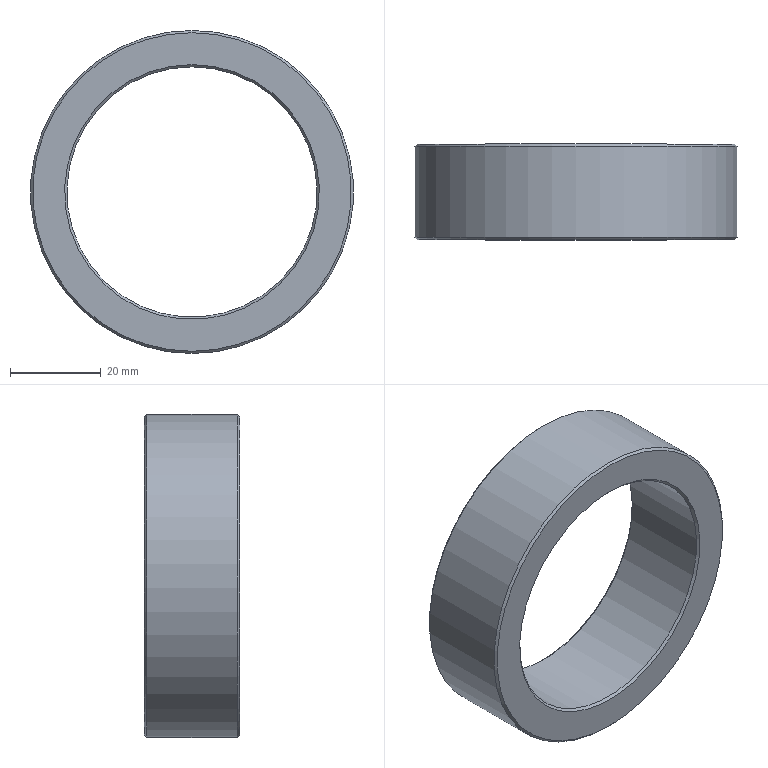Part | NX | features BREP 1, DATUM_CSYS 1 | 1 solid | 8 faces | box 71 x 21 x 71 mm | volume 33152 mm3 | cone 4 | cylinder 2 | plane 2 | commonest cylinder face diameters 55 x1 71 x1
STEP:
#1=CARTESIAN_POINT('',(363.,179.5,35.5));
#2=VERTEX_POINT('',#1);
#3=CARTESIAN_POINT('',(363.,179.5,0.));
#4=DIRECTION('',(0.,1.,0.));
#5=DIRECTION('',(0.,0.,1.));
#6=AXIS2_PLACEMENT_3D('',#3,#4,#5);
#7=CIRCLE('',#6,35.5);
#8=EDGE_CURVE('',#2,#2,#7,.T.);
#9=ORIENTED_EDGE('',*,*,#8,.F.);
#10=EDGE_LOOP('',(#9));
#11=FACE_BOUND('',#10,.T.);
#12=CARTESIAN_POINT('',(363.,159.5,35.5));
#13=VERTEX_POINT('',#12);
#14=CARTESIAN_POINT('',(363.,159.5,0.));
#15=DIRECTION('',(0.,1.,0.));
#16=DIRECTION('',(0.,0.,1.));
#17=AXIS2_PLACEMENT_3D('',#14,#15,#16);
#18=CIRCLE('',#17,35.5);
#19=EDGE_CURVE('',#13,#13,#18,.T.);
#20=ORIENTED_EDGE('',*,*,#19,.T.);
#21=EDGE_LOOP('',(#20));
#22=FACE_BOUND('',#21,.T.);
#23=CARTESIAN_POINT('',(363.,159.,0.));
#24=DIRECTION('',(0.,1.,0.));
#25=DIRECTION('',(0.,0.,1.));
#26=AXIS2_PLACEMENT_3D('',#23,#24,#25);
#27=CYLINDRICAL_SURFACE('',#26,35.5);
#28=ADVANCED_FACE('',(#11,#22),#27,.T.);
#29=CARTESIAN_POINT('',(363.,180.,35.));
#30=VERTEX_POINT('',#29);
#31=CARTESIAN_POINT('',(363.,180.,0.));
#32=DIRECTION('',(0.,1.,0.));
#33=DIRECTION('',(0.,0.,1.));
#34=AXIS2_PLACEMENT_3D('',#31,#32,#33);
#35=CIRCLE('',#34,35.);
#36=EDGE_CURVE('',#30,#30,#35,.T.);
#37=ORIENTED_EDGE('',*,*,#36,.F.);
#38=EDGE_LOOP('',(#37));
#39=FACE_BOUND('',#38,.T.);
#40=ORIENTED_EDGE('',*,*,#8,.T.);
#41=EDGE_LOOP('',(#40));
#42=FACE_BOUND('',#41,.T.);
#43=CARTESIAN_POINT('',(363.,179.5,0.));
#44=DIRECTION('',(0.,-1.,0.));
#45=DIRECTION('',(0.,0.,-1.));
#46=AXIS2_PLACEMENT_3D('',#43,#44,#45);
#47=CONICAL_SURFACE('',#46,35.5,0.7854);
#48=ADVANCED_FACE('',(#39,#42),#47,.T.);
#49=CARTESIAN_POINT('',(363.,180.,28.));
#50=VERTEX_POINT('',#49);
#51=CARTESIAN_POINT('',(363.,180.,0.));
#52=DIRECTION('',(0.,1.,0.));
#53=DIRECTION('',(0.,0.,1.));
#54=AXIS2_PLACEMENT_3D('',#51,#52,#53);
#55=CIRCLE('',#54,28.);
#56=EDGE_CURVE('',#50,#50,#55,.T.);
#57=ORIENTED_EDGE('',*,*,#56,.F.);
#58=EDGE_LOOP('',(#57));
#59=FACE_BOUND('',#58,.T.);
#60=ORIENTED_EDGE('',*,*,#36,.T.);
#61=EDGE_LOOP('',(#60));
#62=FACE_BOUND('',#61,.T.);
#63=CARTESIAN_POINT('',(328.,180.,0.));
#64=DIRECTION('',(0.,-1.,0.));
#65=DIRECTION('',(0.,0.,-1.));
#66=AXIS2_PLACEMENT_3D('',#63,#64,#65);
#67=PLANE('',#66);
#68=ADVANCED_FACE('',(#59,#62),#67,.F.);
#69=CARTESIAN_POINT('',(363.,179.5,27.5));
#70=VERTEX_POINT('',#69);
#71=CARTESIAN_POINT('',(363.,179.5,0.));
#72=DIRECTION('',(0.,1.,0.));
#73=DIRECTION('',(0.,0.,1.));
#74=AXIS2_PLACEMENT_3D('',#71,#72,#73);
#75=CIRCLE('',#74,27.5);
#76=EDGE_CURVE('',#70,#70,#75,.T.);
#77=ORIENTED_EDGE('',*,*,#76,.F.);
#78=EDGE_LOOP('',(#77));
#79=FACE_BOUND('',#78,.T.);
#80=ORIENTED_EDGE('',*,*,#56,.T.);
#81=EDGE_LOOP('',(#80));
#82=FACE_BOUND('',#81,.T.);
#83=CARTESIAN_POINT('',(363.,180.,0.));
#84=DIRECTION('',(0.,1.,0.));
#85=DIRECTION('',(0.,0.,1.));
#86=AXIS2_PLACEMENT_3D('',#83,#84,#85);
#87=CONICAL_SURFACE('',#86,28.,0.7854);
#88=ADVANCED_FACE('',(#79,#82),#87,.F.);
#89=CARTESIAN_POINT('',(363.,159.5,27.5));
#90=VERTEX_POINT('',#89);
#91=CARTESIAN_POINT('',(363.,159.5,0.));
#92=DIRECTION('',(0.,1.,0.));
#93=DIRECTION('',(0.,0.,1.));
#94=AXIS2_PLACEMENT_3D('',#91,#92,#93);
#95=CIRCLE('',#94,27.5);
#96=EDGE_CURVE('',#90,#90,#95,.T.);
#97=ORIENTED_EDGE('',*,*,#96,.F.);
#98=EDGE_LOOP('',(#97));
#99=FACE_BOUND('',#98,.T.);
#100=ORIENTED_EDGE('',*,*,#76,.T.);
#101=EDGE_LOOP('',(#100));
#102=FACE_BOUND('',#101,.T.);
#103=CARTESIAN_POINT('',(363.,159.,0.));
#104=DIRECTION('',(0.,1.,0.));
#105=DIRECTION('',(0.,0.,1.));
#106=AXIS2_PLACEMENT_3D('',#103,#104,#105);
#107=CYLINDRICAL_SURFACE('',#106,27.5);
#108=ADVANCED_FACE('',(#99,#102),#107,.F.);
#109=CARTESIAN_POINT('',(363.,159.,28.));
#110=VERTEX_POINT('',#109);
#111=CARTESIAN_POINT('',(363.,159.,0.));
#112=DIRECTION('',(0.,1.,0.));
#113=DIRECTION('',(0.,0.,1.));
#114=AXIS2_PLACEMENT_3D('',#111,#112,#113);
#115=CIRCLE('',#114,28.);
#116=EDGE_CURVE('',#110,#110,#115,.T.);
#117=ORIENTED_EDGE('',*,*,#116,.F.);
#118=EDGE_LOOP('',(#117));
#119=FACE_BOUND('',#118,.T.);
#120=ORIENTED_EDGE('',*,*,#96,.T.);
#121=EDGE_LOOP('',(#120));
#122=FACE_BOUND('',#121,.T.);
#123=CARTESIAN_POINT('',(363.,159.5,0.));
#124=DIRECTION('',(0.,-1.,0.));
#125=DIRECTION('',(0.,0.,-1.));
#126=AXIS2_PLACEMENT_3D('',#123,#124,#125);
#127=CONICAL_SURFACE('',#126,27.5,0.7854);
#128=ADVANCED_FACE('',(#119,#122),#127,.F.);
#129=CARTESIAN_POINT('',(363.,159.,35.));
#130=VERTEX_POINT('',#129);
#131=CARTESIAN_POINT('',(363.,159.,0.));
#132=DIRECTION('',(0.,1.,0.));
#133=DIRECTION('',(0.,0.,1.));
#134=AXIS2_PLACEMENT_3D('',#131,#132,#133);
#135=CIRCLE('',#134,35.);
#136=EDGE_CURVE('',#130,#130,#135,.T.);
#137=ORIENTED_EDGE('',*,*,#136,.F.);
#138=EDGE_LOOP('',(#137));
#139=FACE_BOUND('',#138,.T.);
#140=ORIENTED_EDGE('',*,*,#116,.T.);
#141=EDGE_LOOP('',(#140));
#142=FACE_BOUND('',#141,.T.);
#143=CARTESIAN_POINT('',(335.,159.,0.));
#144=DIRECTION('',(0.,1.,0.));
#145=DIRECTION('',(0.,0.,1.));
#146=AXIS2_PLACEMENT_3D('',#143,#144,#145);
#147=PLANE('',#146);
#148=ADVANCED_FACE('',(#139,#142),#147,.F.);
#149=ORIENTED_EDGE('',*,*,#19,.F.);
#150=EDGE_LOOP('',(#149));
#151=FACE_BOUND('',#150,.T.);
#152=ORIENTED_EDGE('',*,*,#136,.T.);
#153=EDGE_LOOP('',(#152));
#154=FACE_BOUND('',#153,.T.);
#155=CARTESIAN_POINT('',(363.,159.,0.));
#156=DIRECTION('',(0.,1.,0.));
#157=DIRECTION('',(0.,0.,1.));
#158=AXIS2_PLACEMENT_3D('',#155,#156,#157);
#159=CONICAL_SURFACE('',#158,35.,0.7854);
#160=ADVANCED_FACE('',(#151,#154),#159,.T.);
#161=CLOSED_SHELL('',(#28,#48,#68,#88,#108,#128,#148,#160));
#162=MANIFOLD_SOLID_BREP('',#161);
#163=(LENGTH_UNIT()NAMED_UNIT(*)SI_UNIT(.MILLI.,.METRE.));
#164=UNCERTAINTY_MEASURE_WITH_UNIT(LENGTH_MEASURE(0.00001),#163,'','');
#165=(NAMED_UNIT(*)PLANE_ANGLE_UNIT()SI_UNIT($,.RADIAN.));
#166=(NAMED_UNIT(*)SI_UNIT($,.STERADIAN.)SOLID_ANGLE_UNIT());
#167=(GEOMETRIC_REPRESENTATION_CONTEXT(3)GLOBAL_UNCERTAINTY_ASSIGNED_CONTEXT((#164))GLOBAL_UNIT_ASSIGNED_CONTEXT((#163,#165,#166))REPRESENTATION_CONTEXT('',''));
#168=ADVANCED_BREP_SHAPE_REPRESENTATION('',(#162),#167);